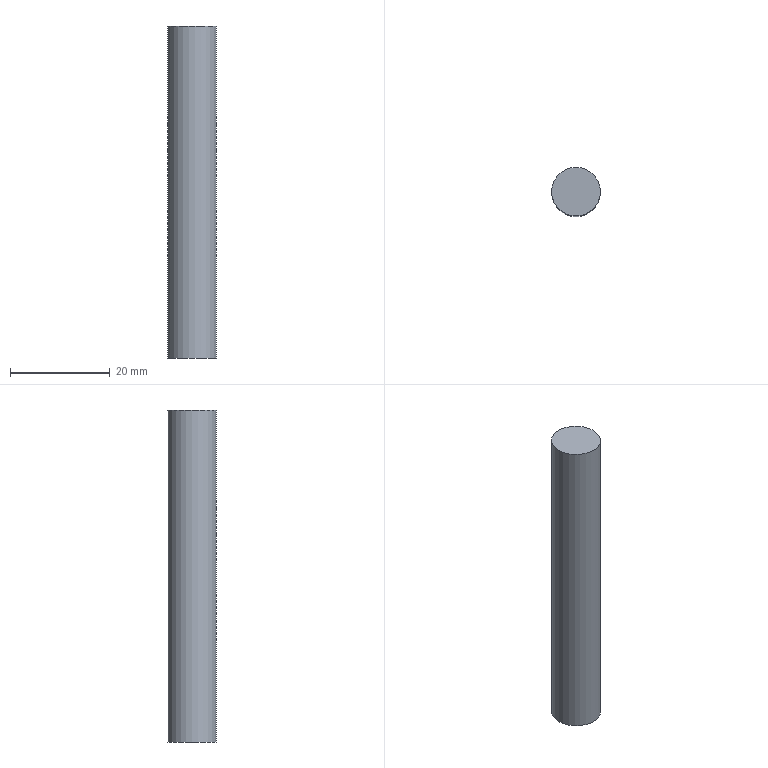Part | NX | features solid 2 | 1 solid | 3 faces | box 9.822 x 9.822 x 66.661 mm | volume 5051 mm3 | plane 2 | cylinder 1 | commonest cylinder face diameters 9.822 x1
STEP:
#1=CARTESIAN_POINT('',(4.911,0.000000344,107.6));
#2=VERTEX_POINT('',#1);
#3=CARTESIAN_POINT('',(-0.00005739,0.000000344,107.6));
#4=DIRECTION('',(0.,0.,-1.));
#5=DIRECTION('',(1.,0.,0.));
#6=AXIS2_PLACEMENT_3D('',#3,#4,#5);
#7=CIRCLE('',#6,4.911);
#8=EDGE_CURVE('',#2,#2,#7,.T.);
#9=ORIENTED_EDGE('',*,*,#8,.F.);
#10=EDGE_LOOP('',(#9));
#11=FACE_BOUND('',#10,.T.);
#12=CARTESIAN_POINT('',(-0.00005739,0.000000344,107.6));
#13=DIRECTION('',(0.,0.,1.));
#14=DIRECTION('',(1.,0.,0.));
#15=AXIS2_PLACEMENT_3D('',#12,#13,#14);
#16=PLANE('',#15);
#17=ADVANCED_FACE('',(#11),#16,.T.);
#18=CARTESIAN_POINT('',(4.911,0.000000344,40.94));
#19=VERTEX_POINT('',#18);
#20=CARTESIAN_POINT('',(-0.00005739,0.000000344,40.94));
#21=DIRECTION('',(0.,0.,1.));
#22=DIRECTION('',(1.,0.,0.));
#23=AXIS2_PLACEMENT_3D('',#20,#21,#22);
#24=CIRCLE('',#23,4.911);
#25=EDGE_CURVE('',#19,#19,#24,.T.);
#26=ORIENTED_EDGE('',*,*,#25,.F.);
#27=EDGE_LOOP('',(#26));
#28=FACE_BOUND('',#27,.T.);
#29=CARTESIAN_POINT('',(-0.00005739,0.000000344,40.94));
#30=DIRECTION('',(0.,0.,-1.));
#31=DIRECTION('',(-1.,0.,0.));
#32=AXIS2_PLACEMENT_3D('',#29,#30,#31);
#33=PLANE('',#32);
#34=ADVANCED_FACE('',(#28),#33,.T.);
#35=ORIENTED_EDGE('',*,*,#8,.T.);
#36=EDGE_LOOP('',(#35));
#37=FACE_BOUND('',#36,.T.);
#38=ORIENTED_EDGE('',*,*,#25,.T.);
#39=EDGE_LOOP('',(#38));
#40=FACE_BOUND('',#39,.T.);
#41=CARTESIAN_POINT('',(-0.00005739,0.000000344,40.94));
#42=DIRECTION('',(0.,0.,1.));
#43=DIRECTION('',(1.,0.,0.));
#44=AXIS2_PLACEMENT_3D('',#41,#42,#43);
#45=CYLINDRICAL_SURFACE('',#44,4.911);
#46=ADVANCED_FACE('',(#37,#40),#45,.T.);
#47=CLOSED_SHELL('',(#17,#34,#46));
#48=MANIFOLD_SOLID_BREP('',#47);
#49=(LENGTH_UNIT()NAMED_UNIT(*)SI_UNIT(.MILLI.,.METRE.));
#50=UNCERTAINTY_MEASURE_WITH_UNIT(LENGTH_MEASURE(0.00001),#49,'','');
#51=(NAMED_UNIT(*)PLANE_ANGLE_UNIT()SI_UNIT($,.RADIAN.));
#52=(NAMED_UNIT(*)SI_UNIT($,.STERADIAN.)SOLID_ANGLE_UNIT());
#53=(GEOMETRIC_REPRESENTATION_CONTEXT(3)GLOBAL_UNCERTAINTY_ASSIGNED_CONTEXT((#50))GLOBAL_UNIT_ASSIGNED_CONTEXT((#49,#51,#52))REPRESENTATION_CONTEXT('',''));
#54=ADVANCED_BREP_SHAPE_REPRESENTATION('',(#48),#53);